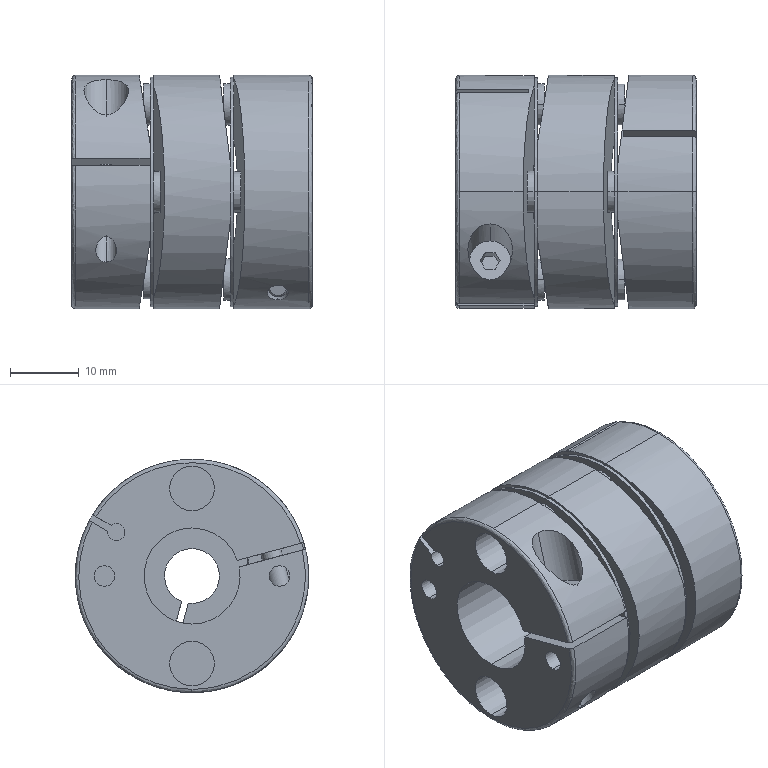Part | SolidWorks | features BaseBody 1 | 1 solid | 171 faces | box 35 x 34 x 34 mm | volume 22881 mm3 | cylinder 82 | plane 78 | spline 7 | cone 4 | commonest cylinder face diameters 3 x20 6 x18 6.5 x12 34 x8 2.5 x6 3.5 x4